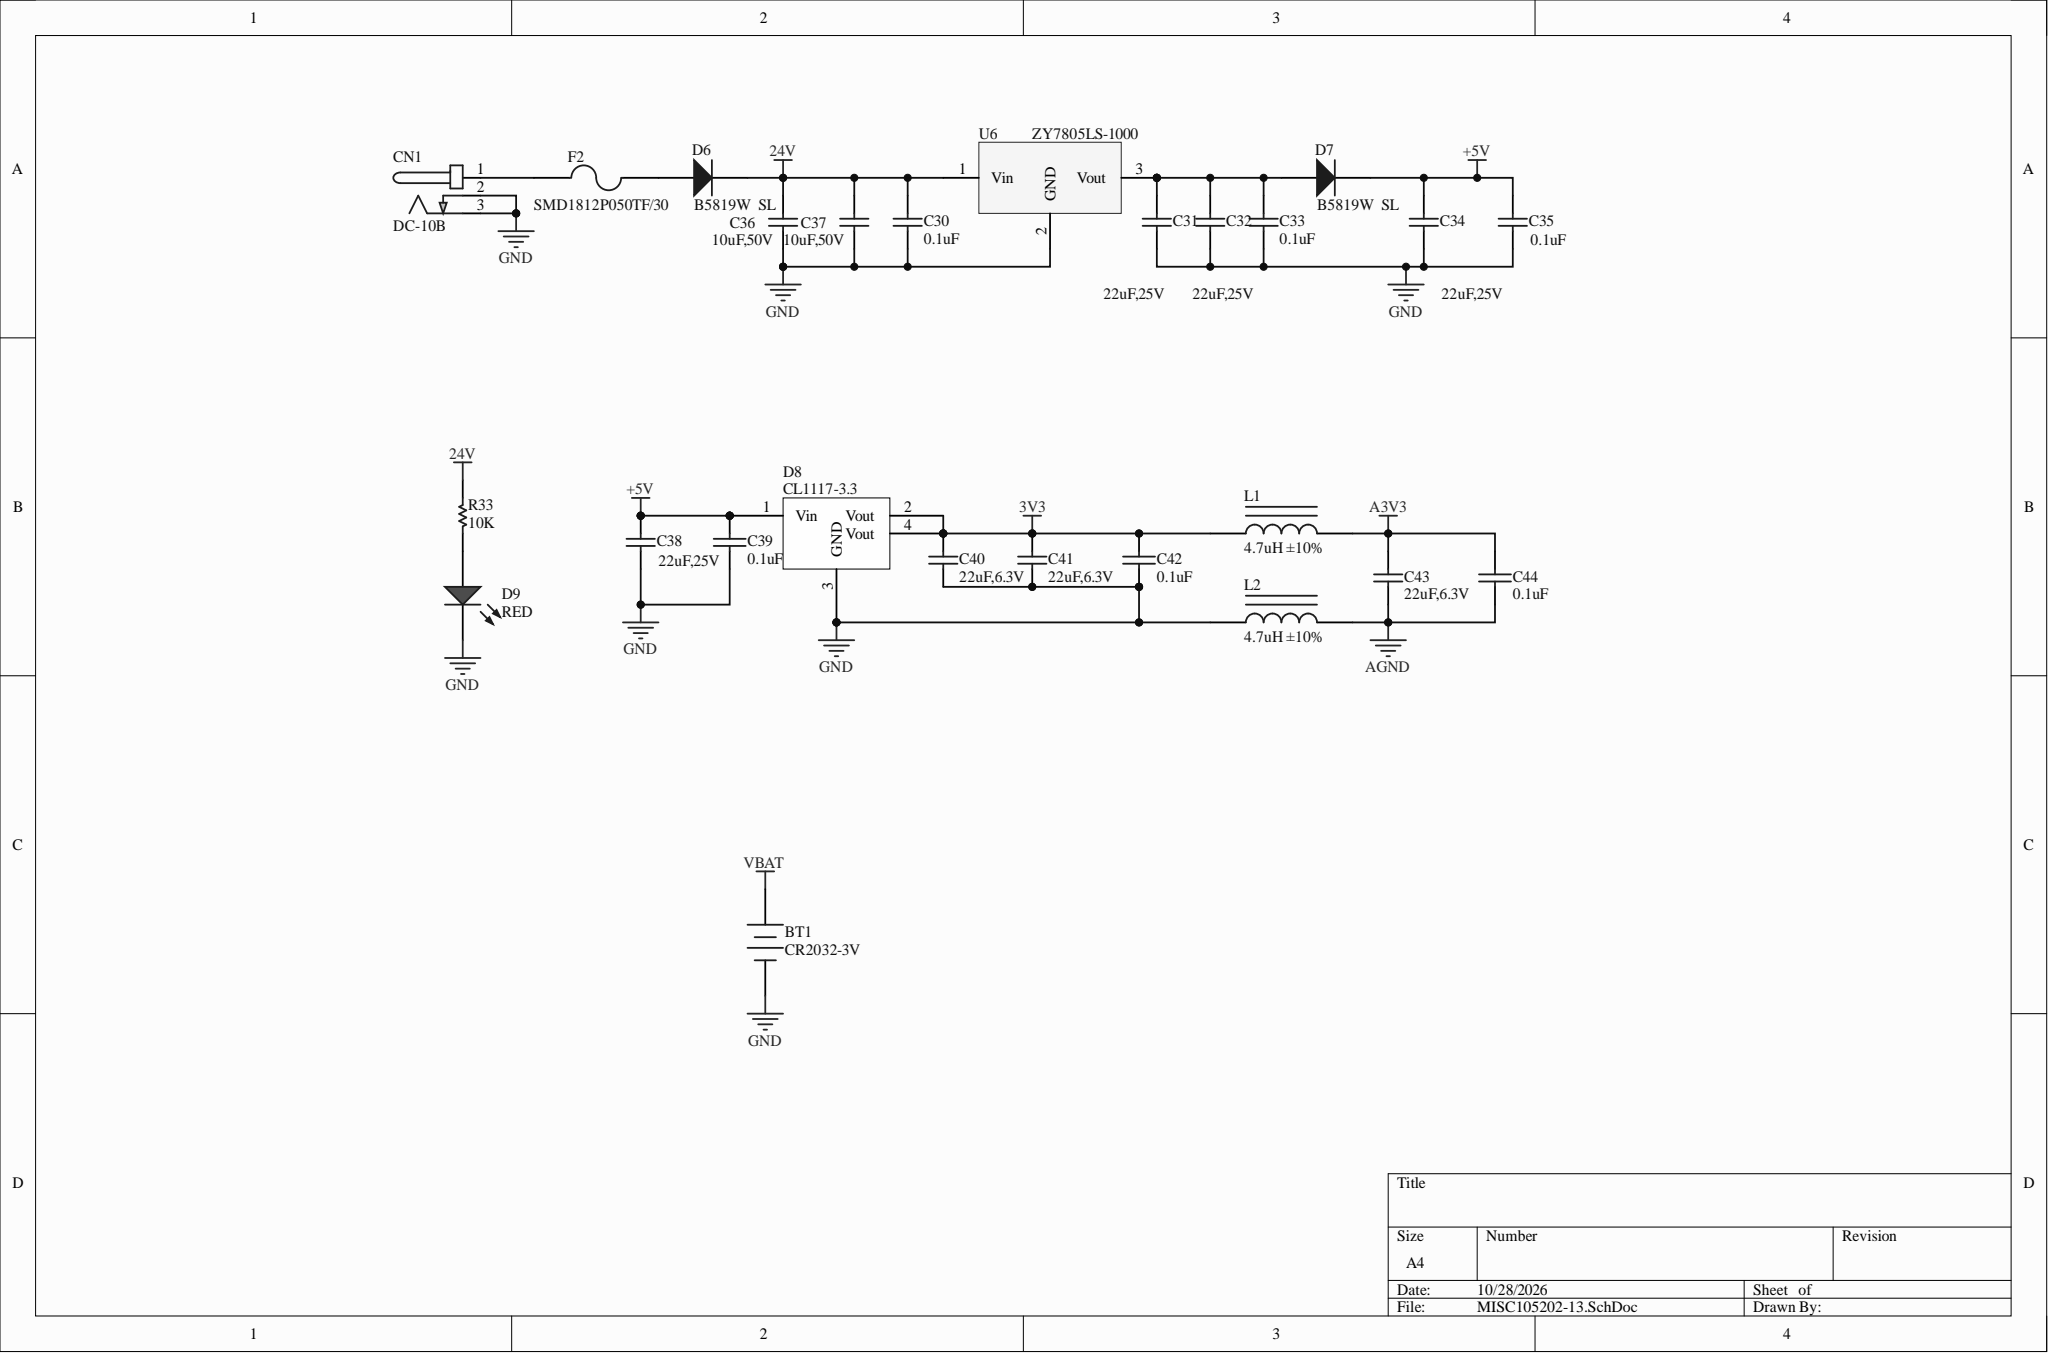Circuit board | Altium Designer | 181 parts | 141 nets | one sheet of the schematic
Parts on this sheet (reference | value | footprint):
BT1 | CR2032-3V | BT1
C30 | 0.1uF | 0402_C
C31 | 22uF,25V | 0805_C
C32 | 22uF,25V | 0805_C
C33 | 0.1uF | 0402_C
C34 | 22uF,25V | 0805_C
C35 | 0.1uF | 0402_C
C36 | 10uF,50V | 1206_C
C37 | 10uF,50V | 1206_C
C38 | 22uF,25V | 0805_C
C39 | 0.1uF | 0603
C40 | 22uF,6.3V | 0603_C
C41 | 22uF,6.3V | 0603_C
C42 | 0.1uF | 0603
C43 | 22uF,6.3V | 0603_C
C44 | 0.1uF | 0603
CN1 | DC-10B | DC10B
D7 | B5819W  SL | SOD-123
D8 | CL1117-3.3 | SOT-223
D9 | RED | 0603_LED_S1
F2 | SMD1812P050TF/30 | 1812
L1 | 4.7uH ±10% | 0603_L
L2 | 4.7uH ±10% | 0603_L
R33 | 10K | 0603
U6 | ZY7805LS-1000 | ZY78xxLS-1000
Nets of these parts (net: part-pin ...):
VBAT: BT1-1
NetD9_A: D9-A R33-2
NetD6_1: F2-1
NetCN1_1: CN1-1 F2-2
NetC31_2: C31-2 C32-2 C33-1 D7-1 U6-3
GND: BT1-2 C30-2 C31-1 C32-1 C33-2 C34-1 C35-2 C36-1 C37-1 C38-1 C39-1 C40-1 C41-1 C42-1 CN1-2 CN1-3 D8-3 D9-K L2-1 U6-2
AIN2: C30-1 C36-2 C37-2 R33-1 U6-1
AGND: C43-1 C44-1 L2-2
A3V3: C43-2 C44-2 L1-2
+5V: C34-2 C35-1 C38-2 C39-2 D7-2 D8-1
3V3: C40-2 C41-2 C42-2 D8-2 D8-4 L1-1